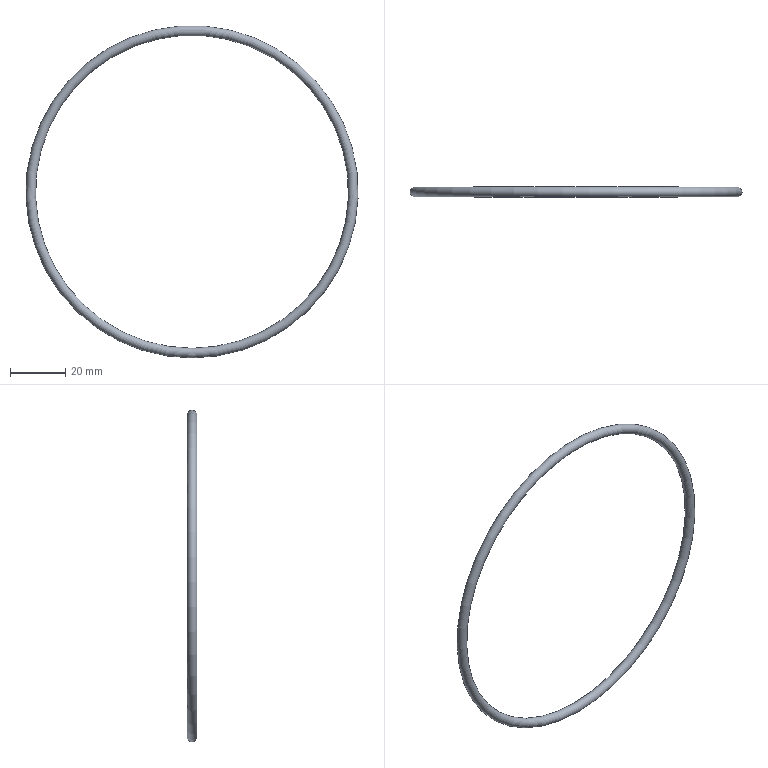Part | NX | features BREP 1 | 1 solid | 1 faces | box 120.7 x 3.5 x 120.7 mm | volume 3542 mm3 | torus 1
STEP:
#1=CARTESIAN_POINT('',(0.,0.,-56.85));
#2=VERTEX_POINT('',#1);
#3=VERTEX_LOOP('',#2);
#4=FACE_BOUND('',#3,.T.);
#5=CARTESIAN_POINT('',(0.,0.,0.));
#6=DIRECTION('',(0.,-1.,0.));
#7=DIRECTION('',(0.,0.,-1.));
#8=AXIS2_PLACEMENT_3D('',#5,#6,#7);
#9=TOROIDAL_SURFACE('',#8,58.6,1.75);
#10=ADVANCED_FACE('',(#4),#9,.T.);
#11=CLOSED_SHELL('',(#10));
#12=MANIFOLD_SOLID_BREP('',#11);
#13=(LENGTH_UNIT()NAMED_UNIT(*)SI_UNIT(.MILLI.,.METRE.));
#14=UNCERTAINTY_MEASURE_WITH_UNIT(LENGTH_MEASURE(0.00001),#13,'','');
#15=(NAMED_UNIT(*)PLANE_ANGLE_UNIT()SI_UNIT($,.RADIAN.));
#16=(NAMED_UNIT(*)SI_UNIT($,.STERADIAN.)SOLID_ANGLE_UNIT());
#17=(GEOMETRIC_REPRESENTATION_CONTEXT(3)GLOBAL_UNCERTAINTY_ASSIGNED_CONTEXT((#14))GLOBAL_UNIT_ASSIGNED_CONTEXT((#13,#15,#16))REPRESENTATION_CONTEXT('',''));
#18=ADVANCED_BREP_SHAPE_REPRESENTATION('',(#12),#17);